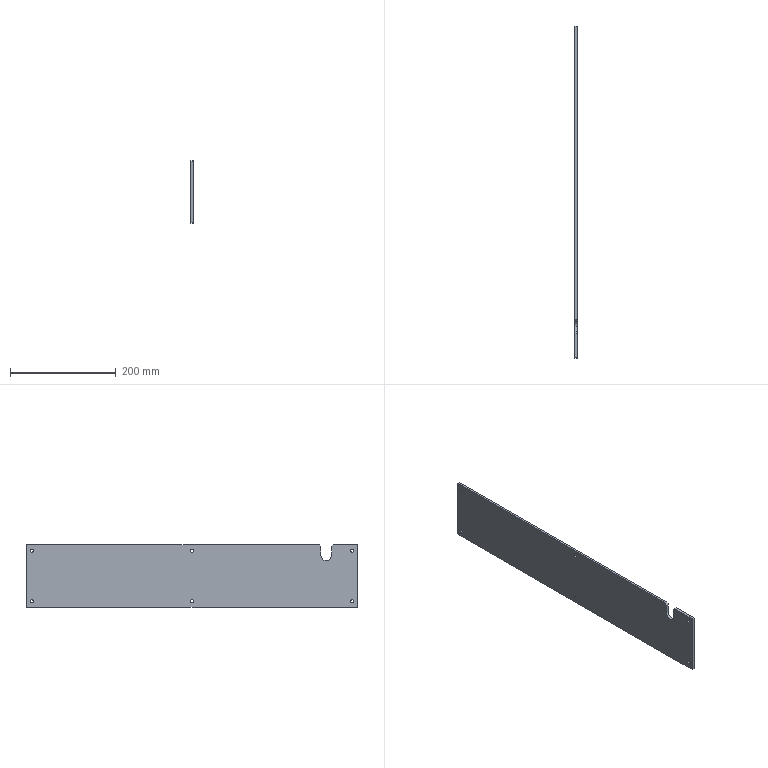Part | SolidWorks | features Chamfer 2, ICE 2, Extrusion 1 | 1 solid | 29 faces | box 5 x 628 x 118 mm | volume 366831 mm3 | plane 15 | cylinder 14 | commonest cylinder face diameters 6 x12 20 x2
STEP:
#1=CARTESIAN_POINT('',(0.,-254.,29.));
#2=VERTEX_POINT('',#1);
#3=CARTESIAN_POINT('',(0.,-244.,39.));
#4=VERTEX_POINT('',#3);
#5=CARTESIAN_POINT('',(0.,-254.,39.));
#6=DIRECTION('',(1.,0.,0.));
#7=DIRECTION('',(0.,0.,-1.));
#8=AXIS2_PLACEMENT_3D('',#5,#6,#7);
#9=CIRCLE('',#8,10.);
#10=EDGE_CURVE('',#2,#4,#9,.T.);
#11=ORIENTED_EDGE('',*,*,#10,.F.);
#12=CARTESIAN_POINT('',(5.,-254.,29.));
#13=VERTEX_POINT('',#12);
#14=CARTESIAN_POINT('',(0.,-254.,29.));
#15=DIRECTION('',(1.,0.,0.));
#16=VECTOR('',#15,1000.);
#17=LINE('',#14,#16);
#18=EDGE_CURVE('',#2,#13,#17,.T.);
#19=ORIENTED_EDGE('',*,*,#18,.T.);
#20=CARTESIAN_POINT('',(5.,-244.,39.));
#21=VERTEX_POINT('',#20);
#22=CARTESIAN_POINT('',(5.,-254.,39.));
#23=DIRECTION('',(1.,0.,0.));
#24=DIRECTION('',(0.,0.,-1.));
#25=AXIS2_PLACEMENT_3D('',#22,#23,#24);
#26=CIRCLE('',#25,10.);
#27=EDGE_CURVE('',#13,#21,#26,.T.);
#28=ORIENTED_EDGE('',*,*,#27,.T.);
#29=CARTESIAN_POINT('',(0.,-244.,39.));
#30=DIRECTION('',(1.,0.,0.));
#31=VECTOR('',#30,1000.);
#32=LINE('',#29,#31);
#33=EDGE_CURVE('',#4,#21,#32,.T.);
#34=ORIENTED_EDGE('',*,*,#33,.F.);
#35=EDGE_LOOP('',(#11,#19,#28,#34));
#36=FACE_OUTER_BOUND('',#35,.T.);
#37=CARTESIAN_POINT('',(0.,-254.,39.));
#38=DIRECTION('',(1.,0.,0.));
#39=DIRECTION('',(0.,0.,-1.));
#40=AXIS2_PLACEMENT_3D('',#37,#38,#39);
#41=CYLINDRICAL_SURFACE('',#40,10.);
#42=ADVANCED_FACE('',(#36),#41,.F.);
#43=CARTESIAN_POINT('',(5.,0.,-51.));
#44=VERTEX_POINT('',#43);
#45=CARTESIAN_POINT('',(5.,0.,-45.));
#46=VERTEX_POINT('',#45);
#47=CARTESIAN_POINT('',(5.,0.,-48.));
#48=DIRECTION('',(-1.,0.,0.));
#49=DIRECTION('',(0.,0.,1.));
#50=AXIS2_PLACEMENT_3D('',#47,#48,#49);
#51=CIRCLE('',#50,3.);
#52=EDGE_CURVE('',#44,#46,#51,.T.);
#53=ORIENTED_EDGE('',*,*,#52,.F.);
#54=CARTESIAN_POINT('',(0.,0.,-51.));
#55=VERTEX_POINT('',#54);
#56=CARTESIAN_POINT('',(5.,0.,-51.));
#57=DIRECTION('',(-1.,0.,0.));
#58=VECTOR('',#57,1000.);
#59=LINE('',#56,#58);
#60=EDGE_CURVE('',#44,#55,#59,.T.);
#61=ORIENTED_EDGE('',*,*,#60,.T.);
#62=CARTESIAN_POINT('',(0.,0.,-45.));
#63=VERTEX_POINT('',#62);
#64=CARTESIAN_POINT('',(0.,0.,-48.));
#65=DIRECTION('',(-1.,0.,0.));
#66=DIRECTION('',(0.,0.,1.));
#67=AXIS2_PLACEMENT_3D('',#64,#65,#66);
#68=CIRCLE('',#67,3.);
#69=EDGE_CURVE('',#55,#63,#68,.T.);
#70=ORIENTED_EDGE('',*,*,#69,.T.);
#71=CARTESIAN_POINT('',(5.,0.,-45.));
#72=DIRECTION('',(-1.,0.,0.));
#73=VECTOR('',#72,1000.);
#74=LINE('',#71,#73);
#75=EDGE_CURVE('',#46,#63,#74,.T.);
#76=ORIENTED_EDGE('',*,*,#75,.F.);
#77=EDGE_LOOP('',(#53,#61,#70,#76));
#78=FACE_OUTER_BOUND('',#77,.T.);
#79=CARTESIAN_POINT('',(5.,0.,-48.));
#80=DIRECTION('',(-1.,0.,0.));
#81=DIRECTION('',(0.,0.,1.));
#82=AXIS2_PLACEMENT_3D('',#79,#80,#81);
#83=CYLINDRICAL_SURFACE('',#82,3.);
#84=ADVANCED_FACE('',(#78),#83,.F.);
#85=CARTESIAN_POINT('',(5.,0.,45.));
#86=VERTEX_POINT('',#85);
#87=CARTESIAN_POINT('',(5.,0.,51.));
#88=VERTEX_POINT('',#87);
#89=CARTESIAN_POINT('',(5.,0.,48.));
#90=DIRECTION('',(-1.,0.,0.));
#91=DIRECTION('',(0.,0.,1.));
#92=AXIS2_PLACEMENT_3D('',#89,#90,#91);
#93=CIRCLE('',#92,3.);
#94=EDGE_CURVE('',#86,#88,#93,.T.);
#95=ORIENTED_EDGE('',*,*,#94,.F.);
#96=CARTESIAN_POINT('',(0.,0.,45.));
#97=VERTEX_POINT('',#96);
#98=CARTESIAN_POINT('',(5.,0.,45.));
#99=DIRECTION('',(-1.,0.,0.));
#100=VECTOR('',#99,1000.);
#101=LINE('',#98,#100);
#102=EDGE_CURVE('',#86,#97,#101,.T.);
#103=ORIENTED_EDGE('',*,*,#102,.T.);
#104=CARTESIAN_POINT('',(0.,0.,51.));
#105=VERTEX_POINT('',#104);
#106=CARTESIAN_POINT('',(0.,0.,48.));
#107=DIRECTION('',(-1.,0.,0.));
#108=DIRECTION('',(0.,0.,1.));
#109=AXIS2_PLACEMENT_3D('',#106,#107,#108);
#110=CIRCLE('',#109,3.);
#111=EDGE_CURVE('',#97,#105,#110,.T.);
#112=ORIENTED_EDGE('',*,*,#111,.T.);
#113=CARTESIAN_POINT('',(5.,0.,51.));
#114=DIRECTION('',(-1.,0.,0.));
#115=VECTOR('',#114,1000.);
#116=LINE('',#113,#115);
#117=EDGE_CURVE('',#88,#105,#116,.T.);
#118=ORIENTED_EDGE('',*,*,#117,.F.);
#119=EDGE_LOOP('',(#95,#103,#112,#118));
#120=FACE_OUTER_BOUND('',#119,.T.);
#121=CARTESIAN_POINT('',(5.,0.,48.));
#122=DIRECTION('',(-1.,0.,0.));
#123=DIRECTION('',(0.,0.,1.));
#124=AXIS2_PLACEMENT_3D('',#121,#122,#123);
#125=CYLINDRICAL_SURFACE('',#124,3.);
#126=ADVANCED_FACE('',(#120),#125,.F.);
#127=CARTESIAN_POINT('',(5.,303.,45.));
#128=VERTEX_POINT('',#127);
#129=CARTESIAN_POINT('',(5.,303.,51.));
#130=VERTEX_POINT('',#129);
#131=CARTESIAN_POINT('',(5.,303.,48.));
#132=DIRECTION('',(-1.,0.,0.));
#133=DIRECTION('',(0.,0.,-1.));
#134=AXIS2_PLACEMENT_3D('',#131,#132,#133);
#135=CIRCLE('',#134,3.);
#136=EDGE_CURVE('',#128,#130,#135,.T.);
#137=ORIENTED_EDGE('',*,*,#136,.F.);
#138=CARTESIAN_POINT('',(0.,303.,45.));
#139=VERTEX_POINT('',#138);
#140=CARTESIAN_POINT('',(5.,303.,45.));
#141=DIRECTION('',(-1.,0.,0.));
#142=VECTOR('',#141,1000.);
#143=LINE('',#140,#142);
#144=EDGE_CURVE('',#128,#139,#143,.T.);
#145=ORIENTED_EDGE('',*,*,#144,.T.);
#146=CARTESIAN_POINT('',(0.,303.,51.));
#147=VERTEX_POINT('',#146);
#148=CARTESIAN_POINT('',(0.,303.,48.));
#149=DIRECTION('',(-1.,0.,0.));
#150=DIRECTION('',(0.,0.,-1.));
#151=AXIS2_PLACEMENT_3D('',#148,#149,#150);
#152=CIRCLE('',#151,3.);
#153=EDGE_CURVE('',#139,#147,#152,.T.);
#154=ORIENTED_EDGE('',*,*,#153,.T.);
#155=CARTESIAN_POINT('',(5.,303.,51.));
#156=DIRECTION('',(-1.,0.,0.));
#157=VECTOR('',#156,1000.);
#158=LINE('',#155,#157);
#159=EDGE_CURVE('',#130,#147,#158,.T.);
#160=ORIENTED_EDGE('',*,*,#159,.F.);
#161=EDGE_LOOP('',(#137,#145,#154,#160));
#162=FACE_OUTER_BOUND('',#161,.T.);
#163=CARTESIAN_POINT('',(5.,303.,48.));
#164=DIRECTION('',(-1.,0.,0.));
#165=DIRECTION('',(0.,0.,1.));
#166=AXIS2_PLACEMENT_3D('',#163,#164,#165);
#167=CYLINDRICAL_SURFACE('',#166,3.);
#168=ADVANCED_FACE('',(#162),#167,.F.);
#169=CARTESIAN_POINT('',(5.,-303.,45.));
#170=VERTEX_POINT('',#169);
#171=CARTESIAN_POINT('',(5.,-303.,51.));
#172=VERTEX_POINT('',#171);
#173=CARTESIAN_POINT('',(5.,-303.,48.));
#174=DIRECTION('',(-1.,0.,0.));
#175=DIRECTION('',(0.,0.,1.));
#176=AXIS2_PLACEMENT_3D('',#173,#174,#175);
#177=CIRCLE('',#176,3.);
#178=EDGE_CURVE('',#170,#172,#177,.T.);
#179=ORIENTED_EDGE('',*,*,#178,.F.);
#180=CARTESIAN_POINT('',(0.,-303.,45.));
#181=VERTEX_POINT('',#180);
#182=CARTESIAN_POINT('',(5.,-303.,45.));
#183=DIRECTION('',(-1.,0.,0.));
#184=VECTOR('',#183,1000.);
#185=LINE('',#182,#184);
#186=EDGE_CURVE('',#170,#181,#185,.T.);
#187=ORIENTED_EDGE('',*,*,#186,.T.);
#188=CARTESIAN_POINT('',(0.,-303.,51.));
#189=VERTEX_POINT('',#188);
#190=CARTESIAN_POINT('',(0.,-303.,48.));
#191=DIRECTION('',(-1.,0.,0.));
#192=DIRECTION('',(0.,0.,1.));
#193=AXIS2_PLACEMENT_3D('',#190,#191,#192);
#194=CIRCLE('',#193,3.);
#195=EDGE_CURVE('',#181,#189,#194,.T.);
#196=ORIENTED_EDGE('',*,*,#195,.T.);
#197=CARTESIAN_POINT('',(5.,-303.,51.));
#198=DIRECTION('',(-1.,0.,0.));
#199=VECTOR('',#198,1000.);
#200=LINE('',#197,#199);
#201=EDGE_CURVE('',#172,#189,#200,.T.);
#202=ORIENTED_EDGE('',*,*,#201,.F.);
#203=EDGE_LOOP('',(#179,#187,#196,#202));
#204=FACE_OUTER_BOUND('',#203,.T.);
#205=CARTESIAN_POINT('',(5.,-303.,48.));
#206=DIRECTION('',(-1.,0.,0.));
#207=DIRECTION('',(0.,0.,1.));
#208=AXIS2_PLACEMENT_3D('',#205,#206,#207);
#209=CYLINDRICAL_SURFACE('',#208,3.);
#210=ADVANCED_FACE('',(#204),#209,.F.);
#211=CARTESIAN_POINT('',(5.,-303.,-51.));
#212=VERTEX_POINT('',#211);
#213=CARTESIAN_POINT('',(5.,-303.,-45.));
#214=VERTEX_POINT('',#213);
#215=CARTESIAN_POINT('',(5.,-303.,-48.));
#216=DIRECTION('',(-1.,0.,0.));
#217=DIRECTION('',(0.,0.,-1.));
#218=AXIS2_PLACEMENT_3D('',#215,#216,#217);
#219=CIRCLE('',#218,3.);
#220=EDGE_CURVE('',#212,#214,#219,.T.);
#221=ORIENTED_EDGE('',*,*,#220,.F.);
#222=CARTESIAN_POINT('',(0.,-303.,-51.));
#223=VERTEX_POINT('',#222);
#224=CARTESIAN_POINT('',(5.,-303.,-51.));
#225=DIRECTION('',(-1.,0.,0.));
#226=VECTOR('',#225,1000.);
#227=LINE('',#224,#226);
#228=EDGE_CURVE('',#212,#223,#227,.T.);
#229=ORIENTED_EDGE('',*,*,#228,.T.);
#230=CARTESIAN_POINT('',(0.,-303.,-45.));
#231=VERTEX_POINT('',#230);
#232=CARTESIAN_POINT('',(0.,-303.,-48.));
#233=DIRECTION('',(-1.,0.,0.));
#234=DIRECTION('',(0.,0.,-1.));
#235=AXIS2_PLACEMENT_3D('',#232,#233,#234);
#236=CIRCLE('',#235,3.);
#237=EDGE_CURVE('',#223,#231,#236,.T.);
#238=ORIENTED_EDGE('',*,*,#237,.T.);
#239=CARTESIAN_POINT('',(5.,-303.,-45.));
#240=DIRECTION('',(-1.,0.,0.));
#241=VECTOR('',#240,1000.);
#242=LINE('',#239,#241);
#243=EDGE_CURVE('',#214,#231,#242,.T.);
#244=ORIENTED_EDGE('',*,*,#243,.F.);
#245=EDGE_LOOP('',(#221,#229,#238,#244));
#246=FACE_OUTER_BOUND('',#245,.T.);
#247=CARTESIAN_POINT('',(5.,-303.,-48.));
#248=DIRECTION('',(-1.,0.,0.));
#249=DIRECTION('',(0.,0.,1.));
#250=AXIS2_PLACEMENT_3D('',#247,#248,#249);
#251=CYLINDRICAL_SURFACE('',#250,3.);
#252=ADVANCED_FACE('',(#246),#251,.F.);
#253=CARTESIAN_POINT('',(5.,303.,-51.));
#254=VERTEX_POINT('',#253);
#255=CARTESIAN_POINT('',(5.,303.,-45.));
#256=VERTEX_POINT('',#255);
#257=CARTESIAN_POINT('',(5.,303.,-48.));
#258=DIRECTION('',(-1.,0.,0.));
#259=DIRECTION('',(0.,0.,1.));
#260=AXIS2_PLACEMENT_3D('',#257,#258,#259);
#261=CIRCLE('',#260,3.);
#262=EDGE_CURVE('',#254,#256,#261,.T.);
#263=ORIENTED_EDGE('',*,*,#262,.F.);
#264=CARTESIAN_POINT('',(0.,303.,-51.));
#265=VERTEX_POINT('',#264);
#266=CARTESIAN_POINT('',(5.,303.,-51.));
#267=DIRECTION('',(-1.,0.,0.));
#268=VECTOR('',#267,1000.);
#269=LINE('',#266,#268);
#270=EDGE_CURVE('',#254,#265,#269,.T.);
#271=ORIENTED_EDGE('',*,*,#270,.T.);
#272=CARTESIAN_POINT('',(0.,303.,-45.));
#273=VERTEX_POINT('',#272);
#274=CARTESIAN_POINT('',(0.,303.,-48.));
#275=DIRECTION('',(-1.,0.,0.));
#276=DIRECTION('',(0.,0.,1.));
#277=AXIS2_PLACEMENT_3D('',#274,#275,#276);
#278=CIRCLE('',#277,3.);
#279=EDGE_CURVE('',#265,#273,#278,.T.);
#280=ORIENTED_EDGE('',*,*,#279,.T.);
#281=CARTESIAN_POINT('',(5.,303.,-45.));
#282=DIRECTION('',(-1.,0.,0.));
#283=VECTOR('',#282,1000.);
#284=LINE('',#281,#283);
#285=EDGE_CURVE('',#256,#273,#284,.T.);
#286=ORIENTED_EDGE('',*,*,#285,.F.);
#287=EDGE_LOOP('',(#263,#271,#280,#286));
#288=FACE_OUTER_BOUND('',#287,.T.);
#289=CARTESIAN_POINT('',(5.,303.,-48.));
#290=DIRECTION('',(-1.,0.,0.));
#291=DIRECTION('',(0.,0.,1.));
#292=AXIS2_PLACEMENT_3D('',#289,#290,#291);
#293=CYLINDRICAL_SURFACE('',#292,3.);
#294=ADVANCED_FACE('',(#288),#293,.F.);
#295=CARTESIAN_POINT('',(5.,-267.,59.));
#296=VERTEX_POINT('',#295);
#297=CARTESIAN_POINT('',(5.,-313.,59.));
#298=VERTEX_POINT('',#297);
#299=CARTESIAN_POINT('',(5.,314.,59.));
#300=DIRECTION('',(0.,-1.,0.));
#301=VECTOR('',#300,1000.);
#302=LINE('',#299,#301);
#303=EDGE_CURVE('',#296,#298,#302,.T.);
#304=ORIENTED_EDGE('',*,*,#303,.F.);
#305=CARTESIAN_POINT('',(0.,-267.,59.));
#306=VERTEX_POINT('',#305);
#307=CARTESIAN_POINT('',(5.,-267.,59.));
#308=DIRECTION('',(-1.,0.,0.));
#309=VECTOR('',#308,1000.);
#310=LINE('',#307,#309);
#311=EDGE_CURVE('',#296,#306,#310,.T.);
#312=ORIENTED_EDGE('',*,*,#311,.T.);
#313=CARTESIAN_POINT('',(0.,-313.,59.));
#314=VERTEX_POINT('',#313);
#315=CARTESIAN_POINT('',(0.,314.,59.));
#316=DIRECTION('',(0.,-1.,0.));
#317=VECTOR('',#316,1000.);
#318=LINE('',#315,#317);
#319=EDGE_CURVE('',#306,#314,#318,.T.);
#320=ORIENTED_EDGE('',*,*,#319,.T.);
#321=CARTESIAN_POINT('',(5.,-313.,59.));
#322=DIRECTION('',(1.,0.,0.));
#323=VECTOR('',#322,1000.);
#324=LINE('',#321,#323);
#325=EDGE_CURVE('',#314,#298,#324,.T.);
#326=ORIENTED_EDGE('',*,*,#325,.T.);
#327=EDGE_LOOP('',(#304,#312,#320,#326));
#328=FACE_OUTER_BOUND('',#327,.T.);
#329=CARTESIAN_POINT('',(5.,314.,59.));
#330=DIRECTION('',(0.,0.,-1.));
#331=DIRECTION('',(0.,1.,0.));
#332=AXIS2_PLACEMENT_3D('',#329,#330,#331);
#333=PLANE('',#332);
#334=ADVANCED_FACE('',(#328),#333,.F.);
#335=CARTESIAN_POINT('',(0.,313.,59.));
#336=VERTEX_POINT('',#335);
#337=CARTESIAN_POINT('',(0.,-241.,59.));
#338=VERTEX_POINT('',#337);
#339=CARTESIAN_POINT('',(0.,314.,59.));
#340=DIRECTION('',(0.,-1.,0.));
#341=VECTOR('',#340,1000.);
#342=LINE('',#339,#341);
#343=EDGE_CURVE('',#336,#338,#342,.T.);
#344=ORIENTED_EDGE('',*,*,#343,.T.);
#345=CARTESIAN_POINT('',(5.,-241.,59.));
#346=VERTEX_POINT('',#345);
#347=CARTESIAN_POINT('',(5.,-241.,59.));
#348=DIRECTION('',(1.,0.,0.));
#349=VECTOR('',#348,1000.);
#350=LINE('',#347,#349);
#351=EDGE_CURVE('',#338,#346,#350,.T.);
#352=ORIENTED_EDGE('',*,*,#351,.T.);
#353=CARTESIAN_POINT('',(5.,313.,59.));
#354=VERTEX_POINT('',#353);
#355=CARTESIAN_POINT('',(5.,314.,59.));
#356=DIRECTION('',(0.,-1.,0.));
#357=VECTOR('',#356,1000.);
#358=LINE('',#355,#357);
#359=EDGE_CURVE('',#354,#346,#358,.T.);
#360=ORIENTED_EDGE('',*,*,#359,.F.);
#361=CARTESIAN_POINT('',(5.,313.,59.));
#362=DIRECTION('',(-1.,0.,0.));
#363=VECTOR('',#362,1000.);
#364=LINE('',#361,#363);
#365=EDGE_CURVE('',#354,#336,#364,.T.);
#366=ORIENTED_EDGE('',*,*,#365,.T.);
#367=EDGE_LOOP('',(#344,#352,#360,#366));
#368=FACE_OUTER_BOUND('',#367,.T.);
#369=CARTESIAN_POINT('',(5.,314.,59.));
#370=DIRECTION('',(0.,0.,-1.));
#371=DIRECTION('',(0.,1.,0.));
#372=AXIS2_PLACEMENT_3D('',#369,#370,#371);
#373=PLANE('',#372);
#374=ADVANCED_FACE('',(#368),#373,.F.);
#375=CARTESIAN_POINT('',(0.,-314.,58.));
#376=VERTEX_POINT('',#375);
#377=CARTESIAN_POINT('',(0.,-314.,-58.));
#378=VERTEX_POINT('',#377);
#379=CARTESIAN_POINT('',(0.,-314.,-59.));
#380=DIRECTION('',(0.,0.,-1.));
#381=VECTOR('',#380,1000.);
#382=LINE('',#379,#381);
#383=EDGE_CURVE('',#376,#378,#382,.T.);
#384=ORIENTED_EDGE('',*,*,#383,.T.);
#385=CARTESIAN_POINT('',(5.,-314.,-58.));
#386=VERTEX_POINT('',#385);
#387=CARTESIAN_POINT('',(5.,-314.,-58.));
#388=DIRECTION('',(1.,0.,0.));
#389=VECTOR('',#388,1000.);
#390=LINE('',#387,#389);
#391=EDGE_CURVE('',#378,#386,#390,.T.);
#392=ORIENTED_EDGE('',*,*,#391,.T.);
#393=CARTESIAN_POINT('',(5.,-314.,58.));
#394=VERTEX_POINT('',#393);
#395=CARTESIAN_POINT('',(5.,-314.,-59.));
#396=DIRECTION('',(0.,0.,-1.));
#397=VECTOR('',#396,1000.);
#398=LINE('',#395,#397);
#399=EDGE_CURVE('',#394,#386,#398,.T.);
#400=ORIENTED_EDGE('',*,*,#399,.F.);
#401=CARTESIAN_POINT('',(5.,-314.,58.));
#402=DIRECTION('',(-1.,0.,0.));
#403=VECTOR('',#402,1000.);
#404=LINE('',#401,#403);
#405=EDGE_CURVE('',#394,#376,#404,.T.);
#406=ORIENTED_EDGE('',*,*,#405,.T.);
#407=EDGE_LOOP('',(#384,#392,#400,#406));
#408=FACE_OUTER_BOUND('',#407,.T.);
#409=CARTESIAN_POINT('',(5.,-314.,-59.));
#410=DIRECTION('',(0.,1.,0.));
#411=DIRECTION('',(0.,0.,1.));
#412=AXIS2_PLACEMENT_3D('',#409,#410,#411);
#413=PLANE('',#412);
#414=ADVANCED_FACE('',(#408),#413,.F.);
#415=CARTESIAN_POINT('',(5.,-313.,-59.));
#416=VERTEX_POINT('',#415);
#417=CARTESIAN_POINT('',(5.,313.,-59.));
#418=VERTEX_POINT('',#417);
#419=CARTESIAN_POINT('',(5.,314.,-59.));
#420=DIRECTION('',(0.,1.,0.));
#421=VECTOR('',#420,1000.);
#422=LINE('',#419,#421);
#423=EDGE_CURVE('',#416,#418,#422,.T.);
#424=ORIENTED_EDGE('',*,*,#423,.F.);
#425=CARTESIAN_POINT('',(0.,-313.,-59.));
#426=VERTEX_POINT('',#425);
#427=CARTESIAN_POINT('',(5.,-313.,-59.));
#428=DIRECTION('',(-1.,0.,0.));
#429=VECTOR('',#428,1000.);
#430=LINE('',#427,#429);
#431=EDGE_CURVE('',#416,#426,#430,.T.);
#432=ORIENTED_EDGE('',*,*,#431,.T.);
#433=CARTESIAN_POINT('',(0.,313.,-59.));
#434=VERTEX_POINT('',#433);
#435=CARTESIAN_POINT('',(0.,314.,-59.));
#436=DIRECTION('',(0.,1.,0.));
#437=VECTOR('',#436,1000.);
#438=LINE('',#435,#437);
#439=EDGE_CURVE('',#426,#434,#438,.T.);
#440=ORIENTED_EDGE('',*,*,#439,.T.);
#441=CARTESIAN_POINT('',(5.,313.,-59.));
#442=DIRECTION('',(1.,0.,0.));
#443=VECTOR('',#442,1000.);
#444=LINE('',#441,#443);
#445=EDGE_CURVE('',#434,#418,#444,.T.);
#446=ORIENTED_EDGE('',*,*,#445,.T.);
#447=EDGE_LOOP('',(#424,#432,#440,#446));
#448=FACE_OUTER_BOUND('',#447,.T.);
#449=CARTESIAN_POINT('',(5.,314.,-59.));
#450=DIRECTION('',(0.,0.,1.));
#451=DIRECTION('',(0.,-1.,0.));
#452=AXIS2_PLACEMENT_3D('',#449,#450,#451);
#453=PLANE('',#452);
#454=ADVANCED_FACE('',(#448),#453,.F.);
#455=CARTESIAN_POINT('',(5.,314.,-58.));
#456=VERTEX_POINT('',#455);
#457=CARTESIAN_POINT('',(5.,314.,58.));
#458=VERTEX_POINT('',#457);
#459=CARTESIAN_POINT('',(5.,314.,-59.));
#460=DIRECTION('',(0.,0.,1.));
#461=VECTOR('',#460,1000.);
#462=LINE('',#459,#461);
#463=EDGE_CURVE('',#456,#458,#462,.T.);
#464=ORIENTED_EDGE('',*,*,#463,.F.);
#465=CARTESIAN_POINT('',(0.,314.,-58.));
#466=VERTEX_POINT('',#465);
#467=CARTESIAN_POINT('',(5.,314.,-58.));
#468=DIRECTION('',(-1.,0.,0.));
#469=VECTOR('',#468,1000.);
#470=LINE('',#467,#469);
#471=EDGE_CURVE('',#456,#466,#470,.T.);
#472=ORIENTED_EDGE('',*,*,#471,.T.);
#473=CARTESIAN_POINT('',(0.,314.,58.));
#474=VERTEX_POINT('',#473);
#475=CARTESIAN_POINT('',(0.,314.,-59.));
#476=DIRECTION('',(0.,0.,1.));
#477=VECTOR('',#476,1000.);
#478=LINE('',#475,#477);
#479=EDGE_CURVE('',#466,#474,#478,.T.);
#480=ORIENTED_EDGE('',*,*,#479,.T.);
#481=CARTESIAN_POINT('',(5.,314.,58.));
#482=DIRECTION('',(1.,0.,0.));
#483=VECTOR('',#482,1000.);
#484=LINE('',#481,#483);
#485=EDGE_CURVE('',#474,#458,#484,.T.);
#486=ORIENTED_EDGE('',*,*,#485,.T.);
#487=EDGE_LOOP('',(#464,#472,#480,#486));
#488=FACE_OUTER_BOUND('',#487,.T.);
#489=CARTESIAN_POINT('',(5.,314.,-59.));
#490=DIRECTION('',(0.,-1.,0.));
#491=DIRECTION('',(0.,0.,-1.));
#492=AXIS2_PLACEMENT_3D('',#489,#490,#491);
#493=PLANE('',#492);
#494=ADVANCED_FACE('',(#488),#493,.F.);
#495=CARTESIAN_POINT('',(5.,0.,-48.));
#496=DIRECTION('',(-1.,0.,0.));
#497=DIRECTION('',(0.,0.,1.));
#498=AXIS2_PLACEMENT_3D('',#495,#496,#497);
#499=CIRCLE('',#498,3.);
#500=EDGE_CURVE('',#46,#44,#499,.T.);
#501=ORIENTED_EDGE('',*,*,#500,.T.);
#502=ORIENTED_EDGE('',*,*,#52,.T.);
#503=EDGE_LOOP('',(#501,#502));
#504=FACE_BOUND('',#503,.T.);
#505=CARTESIAN_POINT('',(5.,0.,48.));
#506=DIRECTION('',(-1.,0.,0.));
#507=DIRECTION('',(0.,0.,1.));
#508=AXIS2_PLACEMENT_3D('',#505,#506,#507);
#509=CIRCLE('',#508,3.);
#510=EDGE_CURVE('',#88,#86,#509,.T.);
#511=ORIENTED_EDGE('',*,*,#510,.T.);
#512=ORIENTED_EDGE('',*,*,#94,.T.);
#513=EDGE_LOOP('',(#511,#512));
#514=FACE_BOUND('',#513,.T.);
#515=CARTESIAN_POINT('',(5.,303.,48.));
#516=DIRECTION('',(-1.,0.,0.));
#517=DIRECTION('',(0.,0.,-1.));
#518=AXIS2_PLACEMENT_3D('',#515,#516,#517);
#519=CIRCLE('',#518,3.);
#520=EDGE_CURVE('',#130,#128,#519,.T.);
#521=ORIENTED_EDGE('',*,*,#520,.T.);
#522=ORIENTED_EDGE('',*,*,#136,.T.);
#523=EDGE_LOOP('',(#521,#522));
#524=FACE_BOUND('',#523,.T.);
#525=CARTESIAN_POINT('',(5.,-303.,48.));
#526=DIRECTION('',(-1.,0.,0.));
#527=DIRECTION('',(0.,0.,1.));
#528=AXIS2_PLACEMENT_3D('',#525,#526,#527);
#529=CIRCLE('',#528,3.);
#530=EDGE_CURVE('',#172,#170,#529,.T.);
#531=ORIENTED_EDGE('',*,*,#530,.T.);
#532=ORIENTED_EDGE('',*,*,#178,.T.);
#533=EDGE_LOOP('',(#531,#532));
#534=FACE_BOUND('',#533,.T.);
#535=CARTESIAN_POINT('',(5.,-303.,-48.));
#536=DIRECTION('',(-1.,0.,0.));
#537=DIRECTION('',(0.,0.,-1.));
#538=AXIS2_PLACEMENT_3D('',#535,#536,#537);
#539=CIRCLE('',#538,3.);
#540=EDGE_CURVE('',#214,#212,#539,.T.);
#541=ORIENTED_EDGE('',*,*,#540,.T.);
#542=ORIENTED_EDGE('',*,*,#220,.T.);
#543=EDGE_LOOP('',(#541,#542));
#544=FACE_BOUND('',#543,.T.);
#545=CARTESIAN_POINT('',(5.,303.,-48.));
#546=DIRECTION('',(-1.,0.,0.));
#547=DIRECTION('',(0.,0.,1.));
#548=AXIS2_PLACEMENT_3D('',#545,#546,#547);
#549=CIRCLE('',#548,3.);
#550=EDGE_CURVE('',#256,#254,#549,.T.);
#551=ORIENTED_EDGE('',*,*,#550,.T.);
#552=ORIENTED_EDGE('',*,*,#262,.T.);
#553=EDGE_LOOP('',(#551,#552));
#554=FACE_BOUND('',#553,.T.);
#555=CARTESIAN_POINT('',(5.,-264.,56.));
#556=VERTEX_POINT('',#555);
#557=CARTESIAN_POINT('',(5.,-264.,39.));
#558=VERTEX_POINT('',#557);
#559=CARTESIAN_POINT('',(5.,-264.,39.));
#560=DIRECTION('',(0.,0.,-1.));
#561=VECTOR('',#560,1000.);
#562=LINE('',#559,#561);
#563=EDGE_CURVE('',#556,#558,#562,.T.);
#564=ORIENTED_EDGE('',*,*,#563,.F.);
#565=CARTESIAN_POINT('',(5.,-264.,56.));
#566=DIRECTION('',(0.,-0.7071,0.7071));
#567=VECTOR('',#566,1000.);
#568=LINE('',#565,#567);
#569=EDGE_CURVE('',#556,#296,#568,.T.);
#570=ORIENTED_EDGE('',*,*,#569,.T.);
#571=ORIENTED_EDGE('',*,*,#303,.T.);
#572=CARTESIAN_POINT('',(5.,-314.,58.));
#573=DIRECTION('',(0.,-0.7071,-0.7071));
#574=VECTOR('',#573,1000.);
#575=LINE('',#572,#574);
#576=EDGE_CURVE('',#298,#394,#575,.T.);
#577=ORIENTED_EDGE('',*,*,#576,.T.);
#578=ORIENTED_EDGE('',*,*,#399,.T.);
#579=CARTESIAN_POINT('',(5.,-313.,-59.));
#580=DIRECTION('',(0.,0.7071,-0.7071));
#581=VECTOR('',#580,1000.);
#582=LINE('',#579,#581);
#583=EDGE_CURVE('',#386,#416,#582,.T.);
#584=ORIENTED_EDGE('',*,*,#583,.T.);
#585=ORIENTED_EDGE('',*,*,#423,.T.);
#586=CARTESIAN_POINT('',(5.,314.,-58.));
#587=DIRECTION('',(0.,0.7071,0.7071));
#588=VECTOR('',#587,1000.);
#589=LINE('',#586,#588);
#590=EDGE_CURVE('',#418,#456,#589,.T.);
#591=ORIENTED_EDGE('',*,*,#590,.T.);
#592=ORIENTED_EDGE('',*,*,#463,.T.);
#593=CARTESIAN_POINT('',(5.,313.,59.));
#594=DIRECTION('',(0.,-0.7071,0.7071));
#595=VECTOR('',#594,1000.);
#596=LINE('',#593,#595);
#597=EDGE_CURVE('',#458,#354,#596,.T.);
#598=ORIENTED_EDGE('',*,*,#597,.T.);
#599=ORIENTED_EDGE('',*,*,#359,.T.);
#600=CARTESIAN_POINT('',(5.,-244.,56.));
#601=VERTEX_POINT('',#600);
#602=CARTESIAN_POINT('',(5.,-241.,59.));
#603=DIRECTION('',(0.,-0.7071,-0.7071));
#604=VECTOR('',#603,1000.);
#605=LINE('',#602,#604);
#606=EDGE_CURVE('',#346,#601,#605,.T.);
#607=ORIENTED_EDGE('',*,*,#606,.T.);
#608=CARTESIAN_POINT('',(5.,-244.,39.));
#609=DIRECTION('',(0.,0.,1.));
#610=VECTOR('',#609,1000.);
#611=LINE('',#608,#610);
#612=EDGE_CURVE('',#21,#601,#611,.T.);
#613=ORIENTED_EDGE('',*,*,#612,.F.);
#614=ORIENTED_EDGE('',*,*,#27,.F.);
#615=CARTESIAN_POINT('',(5.,-254.,39.));
#616=DIRECTION('',(1.,0.,0.));
#617=DIRECTION('',(0.,0.,-1.));
#618=AXIS2_PLACEMENT_3D('',#615,#616,#617);
#619=CIRCLE('',#618,10.);
#620=EDGE_CURVE('',#558,#13,#619,.T.);
#621=ORIENTED_EDGE('',*,*,#620,.F.);
#622=EDGE_LOOP('',(#564,#570,#571,#577,#578,#584,#585,#591,#592,#598,#599,#607,#613,#614,#621));
#623=FACE_OUTER_BOUND('',#622,.T.);
#624=CARTESIAN_POINT('',(5.,-314.,59.));
#625=DIRECTION('',(-1.,0.,0.));
#626=DIRECTION('',(0.,0.,1.));
#627=AXIS2_PLACEMENT_3D('',#624,#625,#626);
#628=PLANE('',#627);
#629=ADVANCED_FACE('',(#504,#514,#524,#534,#544,#554,#623),#628,.F.);
#630=ORIENTED_EDGE('',*,*,#319,.F.);
#631=CARTESIAN_POINT('',(0.,-264.,56.));
#632=VERTEX_POINT('',#631);
#633=CARTESIAN_POINT('',(0.,-290.5,82.5));
#634=DIRECTION('',(0.,0.7071,-0.7071));
#635=VECTOR('',#634,1000.);
#636=LINE('',#633,#635);
#637=EDGE_CURVE('',#306,#632,#636,.T.);
#638=ORIENTED_EDGE('',*,*,#637,.T.);
#639=CARTESIAN_POINT('',(0.,-264.,39.));
#640=VERTEX_POINT('',#639);
#641=CARTESIAN_POINT('',(0.,-264.,39.));
#642=DIRECTION('',(0.,0.,-1.));
#643=VECTOR('',#642,1000.);
#644=LINE('',#641,#643);
#645=EDGE_CURVE('',#632,#640,#644,.T.);
#646=ORIENTED_EDGE('',*,*,#645,.T.);
#647=CARTESIAN_POINT('',(0.,-254.,39.));
#648=DIRECTION('',(1.,0.,0.));
#649=DIRECTION('',(0.,0.,-1.));
#650=AXIS2_PLACEMENT_3D('',#647,#648,#649);
#651=CIRCLE('',#650,10.);
#652=EDGE_CURVE('',#640,#2,#651,.T.);
#653=ORIENTED_EDGE('',*,*,#652,.T.);
#654=ORIENTED_EDGE('',*,*,#10,.T.);
#655=CARTESIAN_POINT('',(0.,-244.,56.));
#656=VERTEX_POINT('',#655);
#657=CARTESIAN_POINT('',(0.,-244.,39.));
#658=DIRECTION('',(0.,0.,1.));
#659=VECTOR('',#658,1000.);
#660=LINE('',#657,#659);
#661=EDGE_CURVE('',#4,#656,#660,.T.);
#662=ORIENTED_EDGE('',*,*,#661,.T.);
#663=CARTESIAN_POINT('',(0.,-277.5,22.5));
#664=DIRECTION('',(0.,0.7071,0.7071));
#665=VECTOR('',#664,1000.);
#666=LINE('',#663,#665);
#667=EDGE_CURVE('',#656,#338,#666,.T.);
#668=ORIENTED_EDGE('',*,*,#667,.T.);
#669=ORIENTED_EDGE('',*,*,#343,.F.);
#670=CARTESIAN_POINT('',(0.,-0.5,372.5));
#671=DIRECTION('',(0.,0.7071,-0.7071));
#672=VECTOR('',#671,1000.);
#673=LINE('',#670,#672);
#674=EDGE_CURVE('',#336,#474,#673,.T.);
#675=ORIENTED_EDGE('',*,*,#674,.T.);
#676=ORIENTED_EDGE('',*,*,#479,.F.);
#677=CARTESIAN_POINT('',(0.,58.5,-313.5));
#678=DIRECTION('',(0.,-0.7071,-0.7071));
#679=VECTOR('',#678,1000.);
#680=LINE('',#677,#679);
#681=EDGE_CURVE('',#466,#434,#680,.T.);
#682=ORIENTED_EDGE('',*,*,#681,.T.);
#683=ORIENTED_EDGE('',*,*,#439,.F.);
#684=CARTESIAN_POINT('',(0.,-372.5,0.5));
#685=DIRECTION('',(0.,-0.7071,0.7071));
#686=VECTOR('',#685,1000.);
#687=LINE('',#684,#686);
#688=EDGE_CURVE('',#426,#378,#687,.T.);
#689=ORIENTED_EDGE('',*,*,#688,.T.);
#690=ORIENTED_EDGE('',*,*,#383,.F.);
#691=CARTESIAN_POINT('',(0.,-313.5,58.5));
#692=DIRECTION('',(0.,0.7071,0.7071));
#693=VECTOR('',#692,1000.);
#694=LINE('',#691,#693);
#695=EDGE_CURVE('',#376,#314,#694,.T.);
#696=ORIENTED_EDGE('',*,*,#695,.T.);
#697=EDGE_LOOP('',(#630,#638,#646,#653,#654,#662,#668,#669,#675,#676,#682,#683,#689,#690,#696));
#698=FACE_OUTER_BOUND('',#697,.T.);
#699=CARTESIAN_POINT('',(0.,0.,-48.));
#700=DIRECTION('',(-1.,0.,0.));
#701=DIRECTION('',(0.,0.,1.));
#702=AXIS2_PLACEMENT_3D('',#699,#700,#701);
#703=CIRCLE('',#702,3.);
#704=EDGE_CURVE('',#63,#55,#703,.T.);
#705=ORIENTED_EDGE('',*,*,#704,.F.);
#706=ORIENTED_EDGE('',*,*,#69,.F.);
#707=EDGE_LOOP('',(#705,#706));
#708=FACE_BOUND('',#707,.T.);
#709=CARTESIAN_POINT('',(0.,0.,48.));
#710=DIRECTION('',(-1.,0.,0.));
#711=DIRECTION('',(0.,0.,1.));
#712=AXIS2_PLACEMENT_3D('',#709,#710,#711);
#713=CIRCLE('',#712,3.);
#714=EDGE_CURVE('',#105,#97,#713,.T.);
#715=ORIENTED_EDGE('',*,*,#714,.F.);
#716=ORIENTED_EDGE('',*,*,#111,.F.);
#717=EDGE_LOOP('',(#715,#716));
#718=FACE_BOUND('',#717,.T.);
#719=CARTESIAN_POINT('',(0.,303.,48.));
#720=DIRECTION('',(-1.,0.,0.));
#721=DIRECTION('',(0.,0.,-1.));
#722=AXIS2_PLACEMENT_3D('',#719,#720,#721);
#723=CIRCLE('',#722,3.);
#724=EDGE_CURVE('',#147,#139,#723,.T.);
#725=ORIENTED_EDGE('',*,*,#724,.F.);
#726=ORIENTED_EDGE('',*,*,#153,.F.);
#727=EDGE_LOOP('',(#725,#726));
#728=FACE_BOUND('',#727,.T.);
#729=CARTESIAN_POINT('',(0.,-303.,48.));
#730=DIRECTION('',(-1.,0.,0.));
#731=DIRECTION('',(0.,0.,1.));
#732=AXIS2_PLACEMENT_3D('',#729,#730,#731);
#733=CIRCLE('',#732,3.);
#734=EDGE_CURVE('',#189,#181,#733,.T.);
#735=ORIENTED_EDGE('',*,*,#734,.F.);
#736=ORIENTED_EDGE('',*,*,#195,.F.);
#737=EDGE_LOOP('',(#735,#736));
#738=FACE_BOUND('',#737,.T.);
#739=CARTESIAN_POINT('',(0.,-303.,-48.));
#740=DIRECTION('',(-1.,0.,0.));
#741=DIRECTION('',(0.,0.,-1.));
#742=AXIS2_PLACEMENT_3D('',#739,#740,#741);
#743=CIRCLE('',#742,3.);
#744=EDGE_CURVE('',#231,#223,#743,.T.);
#745=ORIENTED_EDGE('',*,*,#744,.F.);
#746=ORIENTED_EDGE('',*,*,#237,.F.);
#747=EDGE_LOOP('',(#745,#746));
#748=FACE_BOUND('',#747,.T.);
#749=CARTESIAN_POINT('',(0.,303.,-48.));
#750=DIRECTION('',(-1.,0.,0.));
#751=DIRECTION('',(0.,0.,1.));
#752=AXIS2_PLACEMENT_3D('',#749,#750,#751);
#753=CIRCLE('',#752,3.);
#754=EDGE_CURVE('',#273,#265,#753,.T.);
#755=ORIENTED_EDGE('',*,*,#754,.F.);
#756=ORIENTED_EDGE('',*,*,#279,.F.);
#757=EDGE_LOOP('',(#755,#756));
#758=FACE_BOUND('',#757,.T.);
#759=CARTESIAN_POINT('',(0.,-314.,59.));
#760=DIRECTION('',(-1.,0.,0.));
#761=DIRECTION('',(0.,0.,1.));
#762=AXIS2_PLACEMENT_3D('',#759,#760,#761);
#763=PLANE('',#762);
#764=ADVANCED_FACE('',(#698,#708,#718,#728,#738,#748,#758),#763,.T.);
#765=ORIENTED_EDGE('',*,*,#583,.F.);
#766=ORIENTED_EDGE('',*,*,#391,.F.);
#767=ORIENTED_EDGE('',*,*,#688,.F.);
#768=ORIENTED_EDGE('',*,*,#431,.F.);
#769=EDGE_LOOP('',(#765,#766,#767,#768));
#770=FACE_OUTER_BOUND('',#769,.T.);
#771=CARTESIAN_POINT('',(5.,-313.,-59.));
#772=DIRECTION('',(0.,0.7071,0.7071));
#773=DIRECTION('',(0.,-0.7071,0.7071));
#774=AXIS2_PLACEMENT_3D('',#771,#772,#773);
#775=PLANE('',#774);
#776=ADVANCED_FACE('',(#770),#775,.F.);
#777=ORIENTED_EDGE('',*,*,#576,.F.);
#778=ORIENTED_EDGE('',*,*,#325,.F.);
#779=ORIENTED_EDGE('',*,*,#695,.F.);
#780=ORIENTED_EDGE('',*,*,#405,.F.);
#781=EDGE_LOOP('',(#777,#778,#779,#780));
#782=FACE_OUTER_BOUND('',#781,.T.);
#783=CARTESIAN_POINT('',(5.,-314.,58.));
#784=DIRECTION('',(0.,0.7071,-0.7071));
#785=DIRECTION('',(0.,0.7071,0.7071));
#786=AXIS2_PLACEMENT_3D('',#783,#784,#785);
#787=PLANE('',#786);
#788=ADVANCED_FACE('',(#782),#787,.F.);
#789=ORIENTED_EDGE('',*,*,#590,.F.);
#790=ORIENTED_EDGE('',*,*,#445,.F.);
#791=ORIENTED_EDGE('',*,*,#681,.F.);
#792=ORIENTED_EDGE('',*,*,#471,.F.);
#793=EDGE_LOOP('',(#789,#790,#791,#792));
#794=FACE_OUTER_BOUND('',#793,.T.);
#795=CARTESIAN_POINT('',(5.,314.,-58.));
#796=DIRECTION('',(0.,-0.7071,0.7071));
#797=DIRECTION('',(0.,-0.7071,-0.7071));
#798=AXIS2_PLACEMENT_3D('',#795,#796,#797);
#799=PLANE('',#798);
#800=ADVANCED_FACE('',(#794),#799,.F.);
#801=ORIENTED_EDGE('',*,*,#597,.F.);
#802=ORIENTED_EDGE('',*,*,#485,.F.);
#803=ORIENTED_EDGE('',*,*,#674,.F.);
#804=ORIENTED_EDGE('',*,*,#365,.F.);
#805=EDGE_LOOP('',(#801,#802,#803,#804));
#806=FACE_OUTER_BOUND('',#805,.T.);
#807=CARTESIAN_POINT('',(5.,313.,59.));
#808=DIRECTION('',(0.,-0.7071,-0.7071));
#809=DIRECTION('',(0.,0.7071,-0.7071));
#810=AXIS2_PLACEMENT_3D('',#807,#808,#809);
#811=PLANE('',#810);
#812=ADVANCED_FACE('',(#806),#811,.F.);
#813=ORIENTED_EDGE('',*,*,#270,.F.);
#814=ORIENTED_EDGE('',*,*,#550,.F.);
#815=ORIENTED_EDGE('',*,*,#285,.T.);
#816=ORIENTED_EDGE('',*,*,#754,.T.);
#817=EDGE_LOOP('',(#813,#814,#815,#816));
#818=FACE_OUTER_BOUND('',#817,.T.);
#819=CARTESIAN_POINT('',(5.,303.,-48.));
#820=DIRECTION('',(-1.,0.,0.));
#821=DIRECTION('',(0.,0.,1.));
#822=AXIS2_PLACEMENT_3D('',#819,#820,#821);
#823=CYLINDRICAL_SURFACE('',#822,3.);
#824=ADVANCED_FACE('',(#818),#823,.F.);
#825=ORIENTED_EDGE('',*,*,#228,.F.);
#826=ORIENTED_EDGE('',*,*,#540,.F.);
#827=ORIENTED_EDGE('',*,*,#243,.T.);
#828=ORIENTED_EDGE('',*,*,#744,.T.);
#829=EDGE_LOOP('',(#825,#826,#827,#828));
#830=FACE_OUTER_BOUND('',#829,.T.);
#831=CARTESIAN_POINT('',(5.,-303.,-48.));
#832=DIRECTION('',(-1.,0.,0.));
#833=DIRECTION('',(0.,0.,1.));
#834=AXIS2_PLACEMENT_3D('',#831,#832,#833);
#835=CYLINDRICAL_SURFACE('',#834,3.);
#836=ADVANCED_FACE('',(#830),#835,.F.);
#837=ORIENTED_EDGE('',*,*,#186,.F.);
#838=ORIENTED_EDGE('',*,*,#530,.F.);
#839=ORIENTED_EDGE('',*,*,#201,.T.);
#840=ORIENTED_EDGE('',*,*,#734,.T.);
#841=EDGE_LOOP('',(#837,#838,#839,#840));
#842=FACE_OUTER_BOUND('',#841,.T.);
#843=CARTESIAN_POINT('',(5.,-303.,48.));
#844=DIRECTION('',(-1.,0.,0.));
#845=DIRECTION('',(0.,0.,1.));
#846=AXIS2_PLACEMENT_3D('',#843,#844,#845);
#847=CYLINDRICAL_SURFACE('',#846,3.);
#848=ADVANCED_FACE('',(#842),#847,.F.);
#849=ORIENTED_EDGE('',*,*,#144,.F.);
#850=ORIENTED_EDGE('',*,*,#520,.F.);
#851=ORIENTED_EDGE('',*,*,#159,.T.);
#852=ORIENTED_EDGE('',*,*,#724,.T.);
#853=EDGE_LOOP('',(#849,#850,#851,#852));
#854=FACE_OUTER_BOUND('',#853,.T.);
#855=CARTESIAN_POINT('',(5.,303.,48.));
#856=DIRECTION('',(-1.,0.,0.));
#857=DIRECTION('',(0.,0.,1.));
#858=AXIS2_PLACEMENT_3D('',#855,#856,#857);
#859=CYLINDRICAL_SURFACE('',#858,3.);
#860=ADVANCED_FACE('',(#854),#859,.F.);
#861=ORIENTED_EDGE('',*,*,#102,.F.);
#862=ORIENTED_EDGE('',*,*,#510,.F.);
#863=ORIENTED_EDGE('',*,*,#117,.T.);
#864=ORIENTED_EDGE('',*,*,#714,.T.);
#865=EDGE_LOOP('',(#861,#862,#863,#864));
#866=FACE_OUTER_BOUND('',#865,.T.);
#867=CARTESIAN_POINT('',(5.,0.,48.));
#868=DIRECTION('',(-1.,0.,0.));
#869=DIRECTION('',(0.,0.,1.));
#870=AXIS2_PLACEMENT_3D('',#867,#868,#869);
#871=CYLINDRICAL_SURFACE('',#870,3.);
#872=ADVANCED_FACE('',(#866),#871,.F.);
#873=ORIENTED_EDGE('',*,*,#60,.F.);
#874=ORIENTED_EDGE('',*,*,#500,.F.);
#875=ORIENTED_EDGE('',*,*,#75,.T.);
#876=ORIENTED_EDGE('',*,*,#704,.T.);
#877=EDGE_LOOP('',(#873,#874,#875,#876));
#878=FACE_OUTER_BOUND('',#877,.T.);
#879=CARTESIAN_POINT('',(5.,0.,-48.));
#880=DIRECTION('',(-1.,0.,0.));
#881=DIRECTION('',(0.,0.,1.));
#882=AXIS2_PLACEMENT_3D('',#879,#880,#881);
#883=CYLINDRICAL_SURFACE('',#882,3.);
#884=ADVANCED_FACE('',(#878),#883,.F.);
#885=ORIENTED_EDGE('',*,*,#18,.F.);
#886=ORIENTED_EDGE('',*,*,#652,.F.);
#887=CARTESIAN_POINT('',(0.,-264.,39.));
#888=DIRECTION('',(1.,0.,0.));
#889=VECTOR('',#888,1000.);
#890=LINE('',#887,#889);
#891=EDGE_CURVE('',#640,#558,#890,.T.);
#892=ORIENTED_EDGE('',*,*,#891,.T.);
#893=ORIENTED_EDGE('',*,*,#620,.T.);
#894=EDGE_LOOP('',(#885,#886,#892,#893));
#895=FACE_OUTER_BOUND('',#894,.T.);
#896=CARTESIAN_POINT('',(0.,-254.,39.));
#897=DIRECTION('',(1.,0.,0.));
#898=DIRECTION('',(0.,0.,-1.));
#899=AXIS2_PLACEMENT_3D('',#896,#897,#898);
#900=CYLINDRICAL_SURFACE('',#899,10.);
#901=ADVANCED_FACE('',(#895),#900,.F.);
#902=ORIENTED_EDGE('',*,*,#645,.F.);
#903=CARTESIAN_POINT('',(0.,-264.,56.));
#904=DIRECTION('',(1.,0.,0.));
#905=VECTOR('',#904,1000.);
#906=LINE('',#903,#905);
#907=EDGE_CURVE('',#632,#556,#906,.T.);
#908=ORIENTED_EDGE('',*,*,#907,.T.);
#909=ORIENTED_EDGE('',*,*,#563,.T.);
#910=ORIENTED_EDGE('',*,*,#891,.F.);
#911=EDGE_LOOP('',(#902,#908,#909,#910));
#912=FACE_OUTER_BOUND('',#911,.T.);
#913=CARTESIAN_POINT('',(0.,-264.,39.));
#914=DIRECTION('',(0.,-1.,0.));
#915=DIRECTION('',(1.,0.,0.));
#916=AXIS2_PLACEMENT_3D('',#913,#914,#915);
#917=PLANE('',#916);
#918=ADVANCED_FACE('',(#912),#917,.F.);
#919=ORIENTED_EDGE('',*,*,#612,.T.);
#920=CARTESIAN_POINT('',(0.,-244.,56.));
#921=DIRECTION('',(-1.,0.,0.));
#922=VECTOR('',#921,1000.);
#923=LINE('',#920,#922);
#924=EDGE_CURVE('',#601,#656,#923,.T.);
#925=ORIENTED_EDGE('',*,*,#924,.T.);
#926=ORIENTED_EDGE('',*,*,#661,.F.);
#927=ORIENTED_EDGE('',*,*,#33,.T.);
#928=EDGE_LOOP('',(#919,#925,#926,#927));
#929=FACE_OUTER_BOUND('',#928,.T.);
#930=CARTESIAN_POINT('',(0.,-244.,39.));
#931=DIRECTION('',(0.,1.,0.));
#932=DIRECTION('',(-1.,0.,0.));
#933=AXIS2_PLACEMENT_3D('',#930,#931,#932);
#934=PLANE('',#933);
#935=ADVANCED_FACE('',(#929),#934,.F.);
#936=ORIENTED_EDGE('',*,*,#637,.F.);
#937=ORIENTED_EDGE('',*,*,#311,.F.);
#938=ORIENTED_EDGE('',*,*,#569,.F.);
#939=ORIENTED_EDGE('',*,*,#907,.F.);
#940=EDGE_LOOP('',(#936,#937,#938,#939));
#941=FACE_OUTER_BOUND('',#940,.T.);
#942=CARTESIAN_POINT('',(0.,-264.,56.));
#943=DIRECTION('',(0.,-0.7071,-0.7071));
#944=DIRECTION('',(0.,0.7071,-0.7071));
#945=AXIS2_PLACEMENT_3D('',#942,#943,#944);
#946=PLANE('',#945);
#947=ADVANCED_FACE('',(#941),#946,.F.);
#948=ORIENTED_EDGE('',*,*,#667,.F.);
#949=ORIENTED_EDGE('',*,*,#924,.F.);
#950=ORIENTED_EDGE('',*,*,#606,.F.);
#951=ORIENTED_EDGE('',*,*,#351,.F.);
#952=EDGE_LOOP('',(#948,#949,#950,#951));
#953=FACE_OUTER_BOUND('',#952,.T.);
#954=CARTESIAN_POINT('',(5.,-241.,59.));
#955=DIRECTION('',(0.,0.7071,-0.7071));
#956=DIRECTION('',(0.,0.7071,0.7071));
#957=AXIS2_PLACEMENT_3D('',#954,#955,#956);
#958=PLANE('',#957);
#959=ADVANCED_FACE('',(#953),#958,.F.);
#960=CLOSED_SHELL('',(#42,#84,#126,#168,#210,#252,#294,#334,#374,#414,#454,#494,#629,#764,#776,#788,#800,#812,#824,#836,#848,#860,#872,#884,#901,#918,#935,#947,#959));
#961=MANIFOLD_SOLID_BREP('',#960);
#962=CARTESIAN_POINT('',(0.,0.,0.));
#963=DIRECTION('',(0.,0.,1.));
#964=DIRECTION('',(1.,0.,0.));
#965=AXIS2_PLACEMENT_3D('',#962,#963,#964);
#966=(LENGTH_UNIT()NAMED_UNIT(*)SI_UNIT(.MILLI.,.METRE.));
#967=UNCERTAINTY_MEASURE_WITH_UNIT(LENGTH_MEASURE(0.00001),#966,'','');
#968=(NAMED_UNIT(*)PLANE_ANGLE_UNIT()SI_UNIT($,.RADIAN.));
#969=(NAMED_UNIT(*)SI_UNIT($,.STERADIAN.)SOLID_ANGLE_UNIT());
#970=(GEOMETRIC_REPRESENTATION_CONTEXT(3)GLOBAL_UNCERTAINTY_ASSIGNED_CONTEXT((#967))GLOBAL_UNIT_ASSIGNED_CONTEXT((#966,#968,#969))REPRESENTATION_CONTEXT('',''));
#971=ADVANCED_BREP_SHAPE_REPRESENTATION('',(#961,#965),#970);